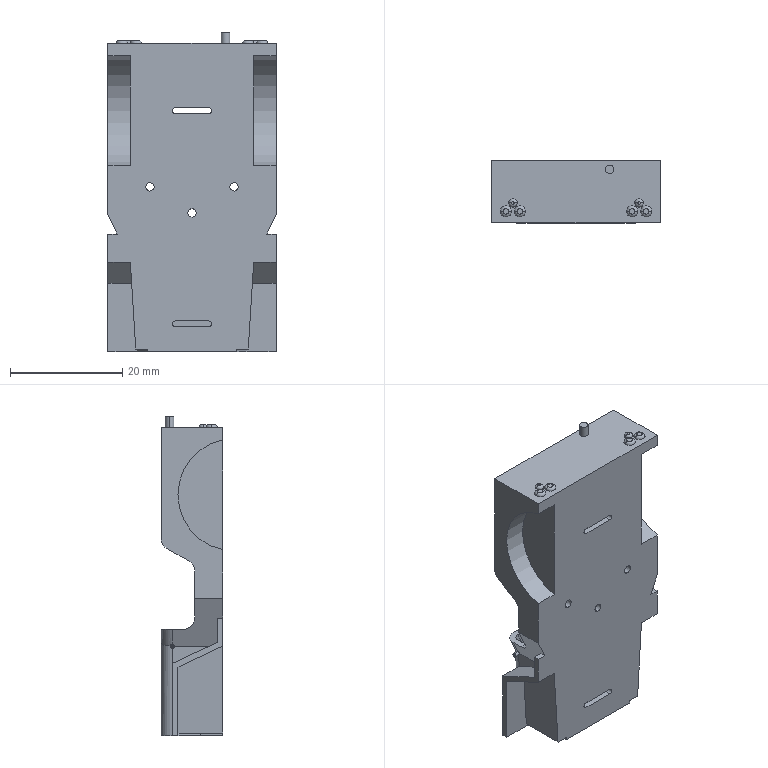Part | SolidWorks | features ICE 10, MirrorPattern 5, Fillet 3, Cut 2, Extrusion 1, Shell 1 | 1 solid | 200 faces | box 30 x 11 x 57 mm | volume 3381 mm3 | plane 114 | cylinder 72 | torus 14 | commonest cylinder face diameters 0.5 x26 4 x10 1 x8 1.5 x8 0.3 x4 0.7 x4